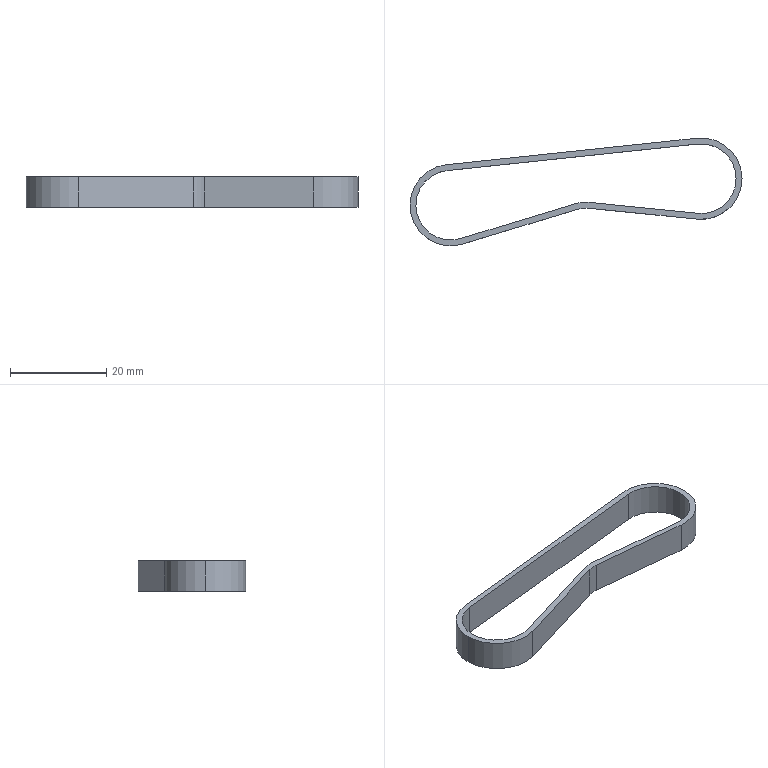Part | NX | features BREP 1 | 1 solid | 16 faces | box 68.88 x 22.38 x 6.4 mm | volume 1208 mm3 | plane 8 | cylinder 8 | commonest cylinder face diameters 14.44 x3 16.88 x3 11.78 x1 14.22 x1
STEP:
#1=CARTESIAN_POINT('',(-23.292,-4.925,-3.2));
#2=VERTEX_POINT('',#1);
#3=CARTESIAN_POINT('',(-0.7189,-7.184,-3.2));
#4=VERTEX_POINT('',#3);
#5=CARTESIAN_POINT('',(-0.7189,-7.184,-3.2));
#6=DIRECTION('',(0.995,-0.09957,0.));
#7=VECTOR('',#6,1000.);
#8=LINE('',#5,#7);
#9=EDGE_CURVE('',#2,#4,#8,.T.);
#10=ORIENTED_EDGE('',*,*,#9,.F.);
#11=CARTESIAN_POINT('',(-23.292,-4.925,3.2));
#12=VERTEX_POINT('',#11);
#13=CARTESIAN_POINT('',(-23.292,-4.925,3.2));
#14=DIRECTION('',(0.,0.,-1.));
#15=VECTOR('',#14,1000.);
#16=LINE('',#13,#15);
#17=EDGE_CURVE('',#12,#2,#16,.T.);
#18=ORIENTED_EDGE('',*,*,#17,.F.);
#19=CARTESIAN_POINT('',(-0.7189,-7.184,3.2));
#20=VERTEX_POINT('',#19);
#21=CARTESIAN_POINT('',(-0.7189,-7.184,3.2));
#22=DIRECTION('',(0.995,-0.09957,0.));
#23=VECTOR('',#22,1000.);
#24=LINE('',#21,#23);
#25=EDGE_CURVE('',#12,#20,#24,.T.);
#26=ORIENTED_EDGE('',*,*,#25,.T.);
#27=CARTESIAN_POINT('',(-0.7189,-7.184,3.2));
#28=DIRECTION('',(0.,0.,-1.));
#29=VECTOR('',#28,1000.);
#30=LINE('',#27,#29);
#31=EDGE_CURVE('',#20,#4,#30,.T.);
#32=ORIENTED_EDGE('',*,*,#31,.T.);
#33=EDGE_LOOP('',(#10,#18,#26,#32));
#34=FACE_BOUND('',#33,.T.);
#35=CARTESIAN_POINT('',(-0.7189,-7.184,3.2));
#36=DIRECTION('',(0.09957,0.995,0.));
#37=DIRECTION('',(-0.995,0.09957,0.));
#38=AXIS2_PLACEMENT_3D('',#35,#36,#37);
#39=PLANE('',#38);
#40=ADVANCED_FACE('',(#34),#39,.T.);
#41=CARTESIAN_POINT('',(-26.059,-5.195,-3.2));
#42=VERTEX_POINT('',#41);
#43=CARTESIAN_POINT('',(-24.,-12.,-3.2));
#44=DIRECTION('',(0.,0.,-1.));
#45=DIRECTION('',(-1.,0.,0.));
#46=AXIS2_PLACEMENT_3D('',#43,#44,#45);
#47=CIRCLE('',#46,7.11);
#48=EDGE_CURVE('',#42,#2,#47,.T.);
#49=ORIENTED_EDGE('',*,*,#48,.F.);
#50=CARTESIAN_POINT('',(-26.059,-5.195,3.2));
#51=VERTEX_POINT('',#50);
#52=CARTESIAN_POINT('',(-26.059,-5.195,3.2));
#53=DIRECTION('',(0.,0.,-1.));
#54=VECTOR('',#53,1000.);
#55=LINE('',#52,#54);
#56=EDGE_CURVE('',#51,#42,#55,.T.);
#57=ORIENTED_EDGE('',*,*,#56,.F.);
#58=CARTESIAN_POINT('',(-24.,-12.,3.2));
#59=DIRECTION('',(0.,0.,-1.));
#60=DIRECTION('',(-1.,0.,0.));
#61=AXIS2_PLACEMENT_3D('',#58,#59,#60);
#62=CIRCLE('',#61,7.11);
#63=EDGE_CURVE('',#51,#12,#62,.T.);
#64=ORIENTED_EDGE('',*,*,#63,.T.);
#65=ORIENTED_EDGE('',*,*,#17,.T.);
#66=EDGE_LOOP('',(#49,#57,#64,#65));
#67=FACE_BOUND('',#66,.T.);
#68=CARTESIAN_POINT('',(-24.,-12.,3.2));
#69=DIRECTION('',(0.,0.,-1.));
#70=DIRECTION('',(-1.,0.,0.));
#71=AXIS2_PLACEMENT_3D('',#68,#69,#70);
#72=CYLINDRICAL_SURFACE('',#71,7.11);
#73=ADVANCED_FACE('',(#67),#72,.T.);
#74=CARTESIAN_POINT('',(-49.909,-12.411,-3.2));
#75=VERTEX_POINT('',#74);
#76=CARTESIAN_POINT('',(-0.7455,2.464,-3.2));
#77=DIRECTION('',(0.9572,0.2896,0.));
#78=VECTOR('',#77,1000.);
#79=LINE('',#76,#78);
#80=EDGE_CURVE('',#75,#42,#79,.T.);
#81=ORIENTED_EDGE('',*,*,#80,.F.);
#82=CARTESIAN_POINT('',(-49.909,-12.411,3.2));
#83=VERTEX_POINT('',#82);
#84=CARTESIAN_POINT('',(-49.909,-12.411,3.2));
#85=DIRECTION('',(0.,0.,-1.));
#86=VECTOR('',#85,1000.);
#87=LINE('',#84,#86);
#88=EDGE_CURVE('',#83,#75,#87,.T.);
#89=ORIENTED_EDGE('',*,*,#88,.F.);
#90=CARTESIAN_POINT('',(-0.7455,2.464,3.2));
#91=DIRECTION('',(0.9572,0.2896,0.));
#92=VECTOR('',#91,1000.);
#93=LINE('',#90,#92);
#94=EDGE_CURVE('',#83,#51,#93,.T.);
#95=ORIENTED_EDGE('',*,*,#94,.T.);
#96=ORIENTED_EDGE('',*,*,#56,.T.);
#97=EDGE_LOOP('',(#81,#89,#95,#96));
#98=FACE_BOUND('',#97,.T.);
#99=CARTESIAN_POINT('',(-0.7455,2.464,3.2));
#100=DIRECTION('',(-0.2896,0.9572,0.));
#101=DIRECTION('',(-0.9572,-0.2896,0.));
#102=AXIS2_PLACEMENT_3D('',#99,#100,#101);
#103=PLANE('',#102);
#104=ADVANCED_FACE('',(#98),#103,.T.);
#105=CARTESIAN_POINT('',(-59.22,-5.5,3.2));
#106=VERTEX_POINT('',#105);
#107=CARTESIAN_POINT('',(-59.22,-5.5,-3.2));
#108=VERTEX_POINT('',#107);
#109=CARTESIAN_POINT('',(-59.22,-5.5,3.2));
#110=DIRECTION('',(0.,0.,-1.));
#111=VECTOR('',#110,1000.);
#112=LINE('',#109,#111);
#113=EDGE_CURVE('',#106,#108,#112,.T.);
#114=ORIENTED_EDGE('',*,*,#113,.F.);
#115=CARTESIAN_POINT('',(-52.,-5.5,3.2));
#116=DIRECTION('',(0.,0.,1.));
#117=DIRECTION('',(-1.,0.,0.));
#118=AXIS2_PLACEMENT_3D('',#115,#116,#117);
#119=CIRCLE('',#118,7.22);
#120=EDGE_CURVE('',#106,#83,#119,.T.);
#121=ORIENTED_EDGE('',*,*,#120,.T.);
#122=ORIENTED_EDGE('',*,*,#88,.T.);
#123=CARTESIAN_POINT('',(-52.,-5.5,-3.2));
#124=DIRECTION('',(0.,0.,1.));
#125=DIRECTION('',(-1.,0.,0.));
#126=AXIS2_PLACEMENT_3D('',#123,#124,#125);
#127=CIRCLE('',#126,7.22);
#128=EDGE_CURVE('',#108,#75,#127,.T.);
#129=ORIENTED_EDGE('',*,*,#128,.F.);
#130=EDGE_LOOP('',(#114,#121,#122,#129));
#131=FACE_BOUND('',#130,.T.);
#132=CARTESIAN_POINT('',(-52.,-5.5,3.2));
#133=DIRECTION('',(0.,0.,-1.));
#134=DIRECTION('',(-1.,0.,0.));
#135=AXIS2_PLACEMENT_3D('',#132,#133,#134);
#136=CYLINDRICAL_SURFACE('',#135,7.22);
#137=ADVANCED_FACE('',(#131),#136,.F.);
#138=CARTESIAN_POINT('',(-0.7594,7.18,-3.2));
#139=VERTEX_POINT('',#138);
#140=CARTESIAN_POINT('',(-52.759,1.68,-3.2));
#141=VERTEX_POINT('',#140);
#142=CARTESIAN_POINT('',(-0.7594,7.18,-3.2));
#143=DIRECTION('',(-0.9945,-0.1052,0.));
#144=VECTOR('',#143,1000.);
#145=LINE('',#142,#144);
#146=EDGE_CURVE('',#139,#141,#145,.T.);
#147=ORIENTED_EDGE('',*,*,#146,.F.);
#148=CARTESIAN_POINT('',(-0.7594,7.18,3.2));
#149=VERTEX_POINT('',#148);
#150=CARTESIAN_POINT('',(-0.7594,7.18,3.2));
#151=DIRECTION('',(0.,0.,-1.));
#152=VECTOR('',#151,1000.);
#153=LINE('',#150,#152);
#154=EDGE_CURVE('',#149,#139,#153,.T.);
#155=ORIENTED_EDGE('',*,*,#154,.F.);
#156=CARTESIAN_POINT('',(-52.759,1.68,3.2));
#157=VERTEX_POINT('',#156);
#158=CARTESIAN_POINT('',(-0.7594,7.18,3.2));
#159=DIRECTION('',(-0.9945,-0.1052,0.));
#160=VECTOR('',#159,1000.);
#161=LINE('',#158,#160);
#162=EDGE_CURVE('',#149,#157,#161,.T.);
#163=ORIENTED_EDGE('',*,*,#162,.T.);
#164=CARTESIAN_POINT('',(-52.759,1.68,3.2));
#165=DIRECTION('',(0.,0.,-1.));
#166=VECTOR('',#165,1000.);
#167=LINE('',#164,#166);
#168=EDGE_CURVE('',#157,#141,#167,.T.);
#169=ORIENTED_EDGE('',*,*,#168,.T.);
#170=EDGE_LOOP('',(#147,#155,#163,#169));
#171=FACE_BOUND('',#170,.T.);
#172=CARTESIAN_POINT('',(-0.7594,7.18,3.2));
#173=DIRECTION('',(0.1052,-0.9945,0.));
#174=DIRECTION('',(0.9945,0.1052,0.));
#175=AXIS2_PLACEMENT_3D('',#172,#173,#174);
#176=PLANE('',#175);
#177=ADVANCED_FACE('',(#171),#176,.T.);
#178=CARTESIAN_POINT('',(0.,0.,-3.2));
#179=DIRECTION('',(0.,0.,1.));
#180=DIRECTION('',(-1.,0.,0.));
#181=AXIS2_PLACEMENT_3D('',#178,#179,#180);
#182=CIRCLE('',#181,7.22);
#183=EDGE_CURVE('',#4,#139,#182,.T.);
#184=ORIENTED_EDGE('',*,*,#183,.F.);
#185=ORIENTED_EDGE('',*,*,#31,.F.);
#186=CARTESIAN_POINT('',(0.,0.,3.2));
#187=DIRECTION('',(0.,0.,1.));
#188=DIRECTION('',(-1.,0.,0.));
#189=AXIS2_PLACEMENT_3D('',#186,#187,#188);
#190=CIRCLE('',#189,7.22);
#191=EDGE_CURVE('',#20,#149,#190,.T.);
#192=ORIENTED_EDGE('',*,*,#191,.T.);
#193=ORIENTED_EDGE('',*,*,#154,.T.);
#194=EDGE_LOOP('',(#184,#185,#192,#193));
#195=FACE_BOUND('',#194,.T.);
#196=CARTESIAN_POINT('',(0.,0.,3.2));
#197=DIRECTION('',(0.,0.,-1.));
#198=DIRECTION('',(-1.,0.,0.));
#199=AXIS2_PLACEMENT_3D('',#196,#197,#198);
#200=CYLINDRICAL_SURFACE('',#199,7.22);
#201=ADVANCED_FACE('',(#195),#200,.F.);
#202=CARTESIAN_POINT('',(-23.414,-6.139,-3.2));
#203=VERTEX_POINT('',#202);
#204=CARTESIAN_POINT('',(-0.8404,-8.398,-3.2));
#205=VERTEX_POINT('',#204);
#206=CARTESIAN_POINT('',(-0.8404,-8.398,-3.2));
#207=DIRECTION('',(0.995,-0.09957,0.));
#208=VECTOR('',#207,1000.);
#209=LINE('',#206,#208);
#210=EDGE_CURVE('',#203,#205,#209,.T.);
#211=ORIENTED_EDGE('',*,*,#210,.T.);
#212=CARTESIAN_POINT('',(-0.8404,-8.398,3.2));
#213=VERTEX_POINT('',#212);
#214=CARTESIAN_POINT('',(-0.8404,-8.398,3.2));
#215=DIRECTION('',(0.,0.,-1.));
#216=VECTOR('',#215,1000.);
#217=LINE('',#214,#216);
#218=EDGE_CURVE('',#213,#205,#217,.T.);
#219=ORIENTED_EDGE('',*,*,#218,.F.);
#220=CARTESIAN_POINT('',(-23.414,-6.139,3.2));
#221=VERTEX_POINT('',#220);
#222=CARTESIAN_POINT('',(-0.8404,-8.398,3.2));
#223=DIRECTION('',(0.995,-0.09957,0.));
#224=VECTOR('',#223,1000.);
#225=LINE('',#222,#224);
#226=EDGE_CURVE('',#221,#213,#225,.T.);
#227=ORIENTED_EDGE('',*,*,#226,.F.);
#228=CARTESIAN_POINT('',(-23.414,-6.139,3.2));
#229=DIRECTION('',(0.,0.,-1.));
#230=VECTOR('',#229,1000.);
#231=LINE('',#228,#230);
#232=EDGE_CURVE('',#221,#203,#231,.T.);
#233=ORIENTED_EDGE('',*,*,#232,.T.);
#234=EDGE_LOOP('',(#211,#219,#227,#233));
#235=FACE_BOUND('',#234,.T.);
#236=CARTESIAN_POINT('',(-0.8404,-8.398,3.2));
#237=DIRECTION('',(0.09957,0.995,0.));
#238=DIRECTION('',(-0.995,0.09957,0.));
#239=AXIS2_PLACEMENT_3D('',#236,#237,#238);
#240=PLANE('',#239);
#241=ADVANCED_FACE('',(#235),#240,.F.);
#242=CARTESIAN_POINT('',(-25.706,-6.362,-3.2));
#243=VERTEX_POINT('',#242);
#244=CARTESIAN_POINT('',(-24.,-12.,-3.2));
#245=DIRECTION('',(0.,0.,-1.));
#246=DIRECTION('',(-1.,0.,0.));
#247=AXIS2_PLACEMENT_3D('',#244,#245,#246);
#248=CIRCLE('',#247,5.89);
#249=EDGE_CURVE('',#243,#203,#248,.T.);
#250=ORIENTED_EDGE('',*,*,#249,.T.);
#251=ORIENTED_EDGE('',*,*,#232,.F.);
#252=CARTESIAN_POINT('',(-25.706,-6.362,3.2));
#253=VERTEX_POINT('',#252);
#254=CARTESIAN_POINT('',(-24.,-12.,3.2));
#255=DIRECTION('',(0.,0.,-1.));
#256=DIRECTION('',(-1.,0.,0.));
#257=AXIS2_PLACEMENT_3D('',#254,#255,#256);
#258=CIRCLE('',#257,5.89);
#259=EDGE_CURVE('',#253,#221,#258,.T.);
#260=ORIENTED_EDGE('',*,*,#259,.F.);
#261=CARTESIAN_POINT('',(-25.706,-6.362,3.2));
#262=DIRECTION('',(0.,0.,-1.));
#263=VECTOR('',#262,1000.);
#264=LINE('',#261,#263);
#265=EDGE_CURVE('',#253,#243,#264,.T.);
#266=ORIENTED_EDGE('',*,*,#265,.T.);
#267=EDGE_LOOP('',(#250,#251,#260,#266));
#268=FACE_BOUND('',#267,.T.);
#269=CARTESIAN_POINT('',(-24.,-12.,3.2));
#270=DIRECTION('',(0.,0.,-1.));
#271=DIRECTION('',(-1.,0.,0.));
#272=AXIS2_PLACEMENT_3D('',#269,#270,#271);
#273=CYLINDRICAL_SURFACE('',#272,5.89);
#274=ADVANCED_FACE('',(#268),#273,.F.);
#275=CARTESIAN_POINT('',(-49.556,-13.578,-3.2));
#276=VERTEX_POINT('',#275);
#277=CARTESIAN_POINT('',(-0.3922,1.296,-3.2));
#278=DIRECTION('',(0.9572,0.2896,0.));
#279=VECTOR('',#278,1000.);
#280=LINE('',#277,#279);
#281=EDGE_CURVE('',#276,#243,#280,.T.);
#282=ORIENTED_EDGE('',*,*,#281,.T.);
#283=ORIENTED_EDGE('',*,*,#265,.F.);
#284=CARTESIAN_POINT('',(-49.556,-13.578,3.2));
#285=VERTEX_POINT('',#284);
#286=CARTESIAN_POINT('',(-0.3922,1.296,3.2));
#287=DIRECTION('',(0.9572,0.2896,0.));
#288=VECTOR('',#287,1000.);
#289=LINE('',#286,#288);
#290=EDGE_CURVE('',#285,#253,#289,.T.);
#291=ORIENTED_EDGE('',*,*,#290,.F.);
#292=CARTESIAN_POINT('',(-49.556,-13.578,3.2));
#293=DIRECTION('',(0.,0.,-1.));
#294=VECTOR('',#293,1000.);
#295=LINE('',#292,#294);
#296=EDGE_CURVE('',#285,#276,#295,.T.);
#297=ORIENTED_EDGE('',*,*,#296,.T.);
#298=EDGE_LOOP('',(#282,#283,#291,#297));
#299=FACE_BOUND('',#298,.T.);
#300=CARTESIAN_POINT('',(-0.3922,1.296,3.2));
#301=DIRECTION('',(-0.2896,0.9572,0.));
#302=DIRECTION('',(-0.9572,-0.2896,0.));
#303=AXIS2_PLACEMENT_3D('',#300,#301,#302);
#304=PLANE('',#303);
#305=ADVANCED_FACE('',(#299),#304,.F.);
#306=CARTESIAN_POINT('',(-60.44,-5.5,3.2));
#307=VERTEX_POINT('',#306);
#308=CARTESIAN_POINT('',(-60.44,-5.5,-3.2));
#309=VERTEX_POINT('',#308);
#310=CARTESIAN_POINT('',(-60.44,-5.5,3.2));
#311=DIRECTION('',(0.,0.,-1.));
#312=VECTOR('',#311,1000.);
#313=LINE('',#310,#312);
#314=EDGE_CURVE('',#307,#309,#313,.T.);
#315=ORIENTED_EDGE('',*,*,#314,.F.);
#316=CARTESIAN_POINT('',(-52.888,2.893,3.2));
#317=VERTEX_POINT('',#316);
#318=CARTESIAN_POINT('',(-52.,-5.5,3.2));
#319=DIRECTION('',(0.,0.,1.));
#320=DIRECTION('',(-1.,0.,0.));
#321=AXIS2_PLACEMENT_3D('',#318,#319,#320);
#322=CIRCLE('',#321,8.44);
#323=EDGE_CURVE('',#317,#307,#322,.T.);
#324=ORIENTED_EDGE('',*,*,#323,.F.);
#325=CARTESIAN_POINT('',(-52.888,2.893,-3.2));
#326=VERTEX_POINT('',#325);
#327=CARTESIAN_POINT('',(-52.888,2.893,3.2));
#328=DIRECTION('',(0.,0.,-1.));
#329=VECTOR('',#328,1000.);
#330=LINE('',#327,#329);
#331=EDGE_CURVE('',#317,#326,#330,.T.);
#332=ORIENTED_EDGE('',*,*,#331,.T.);
#333=CARTESIAN_POINT('',(-52.,-5.5,-3.2));
#334=DIRECTION('',(0.,0.,1.));
#335=DIRECTION('',(-1.,0.,0.));
#336=AXIS2_PLACEMENT_3D('',#333,#334,#335);
#337=CIRCLE('',#336,8.44);
#338=EDGE_CURVE('',#326,#309,#337,.T.);
#339=ORIENTED_EDGE('',*,*,#338,.T.);
#340=EDGE_LOOP('',(#315,#324,#332,#339));
#341=FACE_BOUND('',#340,.T.);
#342=CARTESIAN_POINT('',(-52.,-5.5,3.2));
#343=DIRECTION('',(0.,0.,-1.));
#344=DIRECTION('',(-1.,0.,0.));
#345=AXIS2_PLACEMENT_3D('',#342,#343,#344);
#346=CYLINDRICAL_SURFACE('',#345,8.44);
#347=ADVANCED_FACE('',(#341),#346,.T.);
#348=CARTESIAN_POINT('',(-0.8877,8.393,-3.2));
#349=VERTEX_POINT('',#348);
#350=CARTESIAN_POINT('',(-0.8877,8.393,-3.2));
#351=DIRECTION('',(-0.9945,-0.1052,0.));
#352=VECTOR('',#351,1000.);
#353=LINE('',#350,#352);
#354=EDGE_CURVE('',#349,#326,#353,.T.);
#355=ORIENTED_EDGE('',*,*,#354,.T.);
#356=ORIENTED_EDGE('',*,*,#331,.F.);
#357=CARTESIAN_POINT('',(-0.8877,8.393,3.2));
#358=VERTEX_POINT('',#357);
#359=CARTESIAN_POINT('',(-0.8877,8.393,3.2));
#360=DIRECTION('',(-0.9945,-0.1052,0.));
#361=VECTOR('',#360,1000.);
#362=LINE('',#359,#361);
#363=EDGE_CURVE('',#358,#317,#362,.T.);
#364=ORIENTED_EDGE('',*,*,#363,.F.);
#365=CARTESIAN_POINT('',(-0.8877,8.393,3.2));
#366=DIRECTION('',(0.,0.,-1.));
#367=VECTOR('',#366,1000.);
#368=LINE('',#365,#367);
#369=EDGE_CURVE('',#358,#349,#368,.T.);
#370=ORIENTED_EDGE('',*,*,#369,.T.);
#371=EDGE_LOOP('',(#355,#356,#364,#370));
#372=FACE_BOUND('',#371,.T.);
#373=CARTESIAN_POINT('',(-0.8877,8.393,3.2));
#374=DIRECTION('',(0.1052,-0.9945,0.));
#375=DIRECTION('',(0.9945,0.1052,0.));
#376=AXIS2_PLACEMENT_3D('',#373,#374,#375);
#377=PLANE('',#376);
#378=ADVANCED_FACE('',(#372),#377,.F.);
#379=CARTESIAN_POINT('',(0.,0.,-3.2));
#380=DIRECTION('',(0.,0.,1.));
#381=DIRECTION('',(-1.,0.,0.));
#382=AXIS2_PLACEMENT_3D('',#379,#380,#381);
#383=CIRCLE('',#382,8.44);
#384=EDGE_CURVE('',#205,#349,#383,.T.);
#385=ORIENTED_EDGE('',*,*,#384,.T.);
#386=ORIENTED_EDGE('',*,*,#369,.F.);
#387=CARTESIAN_POINT('',(0.,0.,3.2));
#388=DIRECTION('',(0.,0.,1.));
#389=DIRECTION('',(-1.,0.,0.));
#390=AXIS2_PLACEMENT_3D('',#387,#388,#389);
#391=CIRCLE('',#390,8.44);
#392=EDGE_CURVE('',#213,#358,#391,.T.);
#393=ORIENTED_EDGE('',*,*,#392,.F.);
#394=ORIENTED_EDGE('',*,*,#218,.T.);
#395=EDGE_LOOP('',(#385,#386,#393,#394));
#396=FACE_BOUND('',#395,.T.);
#397=CARTESIAN_POINT('',(0.,0.,3.2));
#398=DIRECTION('',(0.,0.,-1.));
#399=DIRECTION('',(-1.,0.,0.));
#400=AXIS2_PLACEMENT_3D('',#397,#398,#399);
#401=CYLINDRICAL_SURFACE('',#400,8.44);
#402=ADVANCED_FACE('',(#396),#401,.T.);
#403=ORIENTED_EDGE('',*,*,#9,.T.);
#404=ORIENTED_EDGE('',*,*,#183,.T.);
#405=ORIENTED_EDGE('',*,*,#146,.T.);
#406=CARTESIAN_POINT('',(-52.,-5.5,-3.2));
#407=DIRECTION('',(0.,0.,1.));
#408=DIRECTION('',(-1.,0.,0.));
#409=AXIS2_PLACEMENT_3D('',#406,#407,#408);
#410=CIRCLE('',#409,7.22);
#411=EDGE_CURVE('',#141,#108,#410,.T.);
#412=ORIENTED_EDGE('',*,*,#411,.T.);
#413=ORIENTED_EDGE('',*,*,#128,.T.);
#414=ORIENTED_EDGE('',*,*,#80,.T.);
#415=ORIENTED_EDGE('',*,*,#48,.T.);
#416=EDGE_LOOP('',(#403,#404,#405,#412,#413,#414,#415));
#417=FACE_BOUND('',#416,.T.);
#418=ORIENTED_EDGE('',*,*,#384,.F.);
#419=ORIENTED_EDGE('',*,*,#210,.F.);
#420=ORIENTED_EDGE('',*,*,#249,.F.);
#421=ORIENTED_EDGE('',*,*,#281,.F.);
#422=CARTESIAN_POINT('',(-52.,-5.5,-3.2));
#423=DIRECTION('',(0.,0.,1.));
#424=DIRECTION('',(-1.,0.,0.));
#425=AXIS2_PLACEMENT_3D('',#422,#423,#424);
#426=CIRCLE('',#425,8.44);
#427=EDGE_CURVE('',#309,#276,#426,.T.);
#428=ORIENTED_EDGE('',*,*,#427,.F.);
#429=ORIENTED_EDGE('',*,*,#338,.F.);
#430=ORIENTED_EDGE('',*,*,#354,.F.);
#431=EDGE_LOOP('',(#418,#419,#420,#421,#428,#429,#430));
#432=FACE_BOUND('',#431,.T.);
#433=CARTESIAN_POINT('',(0.,0.,-3.2));
#434=DIRECTION('',(0.,0.,-1.));
#435=DIRECTION('',(-1.,0.,0.));
#436=AXIS2_PLACEMENT_3D('',#433,#434,#435);
#437=PLANE('',#436);
#438=ADVANCED_FACE('',(#417,#432),#437,.T.);
#439=ORIENTED_EDGE('',*,*,#191,.F.);
#440=ORIENTED_EDGE('',*,*,#25,.F.);
#441=ORIENTED_EDGE('',*,*,#63,.F.);
#442=ORIENTED_EDGE('',*,*,#94,.F.);
#443=ORIENTED_EDGE('',*,*,#120,.F.);
#444=CARTESIAN_POINT('',(-52.,-5.5,3.2));
#445=DIRECTION('',(0.,0.,1.));
#446=DIRECTION('',(-1.,0.,0.));
#447=AXIS2_PLACEMENT_3D('',#444,#445,#446);
#448=CIRCLE('',#447,7.22);
#449=EDGE_CURVE('',#157,#106,#448,.T.);
#450=ORIENTED_EDGE('',*,*,#449,.F.);
#451=ORIENTED_EDGE('',*,*,#162,.F.);
#452=EDGE_LOOP('',(#439,#440,#441,#442,#443,#450,#451));
#453=FACE_BOUND('',#452,.T.);
#454=ORIENTED_EDGE('',*,*,#392,.T.);
#455=ORIENTED_EDGE('',*,*,#363,.T.);
#456=ORIENTED_EDGE('',*,*,#323,.T.);
#457=CARTESIAN_POINT('',(-52.,-5.5,3.2));
#458=DIRECTION('',(0.,0.,1.));
#459=DIRECTION('',(-1.,0.,0.));
#460=AXIS2_PLACEMENT_3D('',#457,#458,#459);
#461=CIRCLE('',#460,8.44);
#462=EDGE_CURVE('',#307,#285,#461,.T.);
#463=ORIENTED_EDGE('',*,*,#462,.T.);
#464=ORIENTED_EDGE('',*,*,#290,.T.);
#465=ORIENTED_EDGE('',*,*,#259,.T.);
#466=ORIENTED_EDGE('',*,*,#226,.T.);
#467=EDGE_LOOP('',(#454,#455,#456,#463,#464,#465,#466));
#468=FACE_BOUND('',#467,.T.);
#469=CARTESIAN_POINT('',(0.,0.,3.2));
#470=DIRECTION('',(0.,0.,-1.));
#471=DIRECTION('',(-1.,0.,0.));
#472=AXIS2_PLACEMENT_3D('',#469,#470,#471);
#473=PLANE('',#472);
#474=ADVANCED_FACE('',(#453,#468),#473,.F.);
#475=ORIENTED_EDGE('',*,*,#462,.F.);
#476=ORIENTED_EDGE('',*,*,#314,.T.);
#477=ORIENTED_EDGE('',*,*,#427,.T.);
#478=ORIENTED_EDGE('',*,*,#296,.F.);
#479=EDGE_LOOP('',(#475,#476,#477,#478));
#480=FACE_BOUND('',#479,.T.);
#481=CARTESIAN_POINT('',(-52.,-5.5,3.2));
#482=DIRECTION('',(0.,0.,-1.));
#483=DIRECTION('',(-1.,0.,0.));
#484=AXIS2_PLACEMENT_3D('',#481,#482,#483);
#485=CYLINDRICAL_SURFACE('',#484,8.44);
#486=ADVANCED_FACE('',(#480),#485,.T.);
#487=ORIENTED_EDGE('',*,*,#449,.T.);
#488=ORIENTED_EDGE('',*,*,#113,.T.);
#489=ORIENTED_EDGE('',*,*,#411,.F.);
#490=ORIENTED_EDGE('',*,*,#168,.F.);
#491=EDGE_LOOP('',(#487,#488,#489,#490));
#492=FACE_BOUND('',#491,.T.);
#493=CARTESIAN_POINT('',(-52.,-5.5,3.2));
#494=DIRECTION('',(0.,0.,-1.));
#495=DIRECTION('',(-1.,0.,0.));
#496=AXIS2_PLACEMENT_3D('',#493,#494,#495);
#497=CYLINDRICAL_SURFACE('',#496,7.22);
#498=ADVANCED_FACE('',(#492),#497,.F.);
#499=CLOSED_SHELL('',(#40,#73,#104,#137,#177,#201,#241,#274,#305,#347,#378,#402,#438,#474,#486,#498));
#500=MANIFOLD_SOLID_BREP('',#499);
#501=(LENGTH_UNIT()NAMED_UNIT(*)SI_UNIT(.MILLI.,.METRE.));
#502=UNCERTAINTY_MEASURE_WITH_UNIT(LENGTH_MEASURE(0.00001),#501,'','');
#503=(NAMED_UNIT(*)PLANE_ANGLE_UNIT()SI_UNIT($,.RADIAN.));
#504=(NAMED_UNIT(*)SI_UNIT($,.STERADIAN.)SOLID_ANGLE_UNIT());
#505=(GEOMETRIC_REPRESENTATION_CONTEXT(3)GLOBAL_UNCERTAINTY_ASSIGNED_CONTEXT((#502))GLOBAL_UNIT_ASSIGNED_CONTEXT((#501,#503,#504))REPRESENTATION_CONTEXT('',''));
#506=ADVANCED_BREP_SHAPE_REPRESENTATION('',(#500),#505);